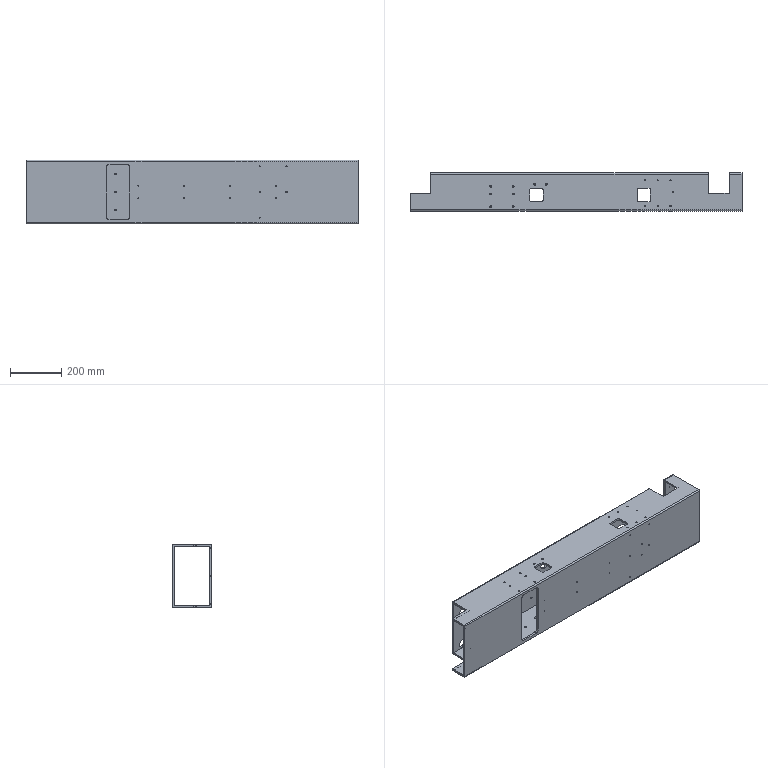Part | SolidWorks | features HoleWzd 10, ICE 9, Fillet 5, Cut 4, MoveFace 4, Extrusion 1 | 1 solid | 261 faces | box 1300 x 150 x 250 mm | volume 6899241 mm3 | cylinder 202 | plane 49 | cone 10 | commonest cylinder face diameters 4.2 x72 6.8 x46 10 x22 8.5 x16 35 x16 20 x12